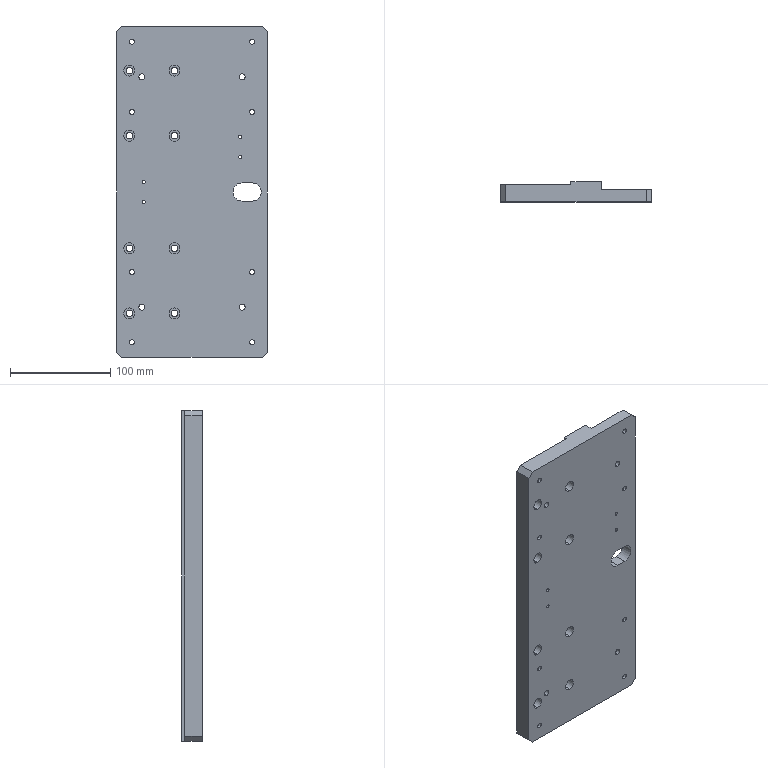Part | SolidWorks | features HoleWzd 5, Cut 3, Chamfer 1, Extrusion 1 | 1 solid | 90 faces | box 150 x 20 x 330 mm | volume 769710 mm3 | cylinder 66 | plane 24 | commonest cylinder face diameters 5 x16 6.6 x16 11 x16 3.3 x8 6 x8 18.2 x2